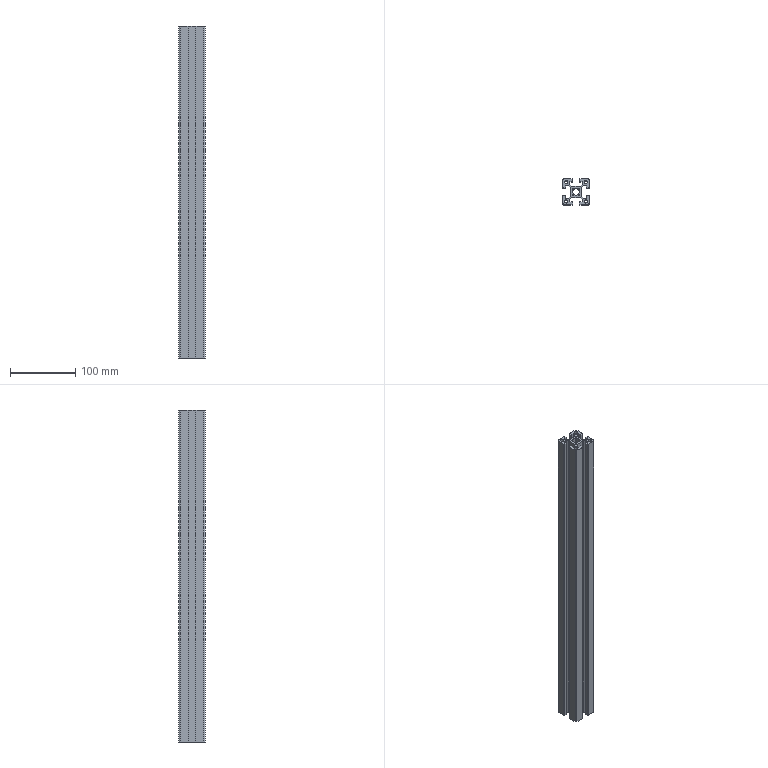Part | SolidWorks | features Extrusion 1 | 1 solid | 125 faces | box 40 x 40 x 510 mm | volume 357748 mm3 | plane 74 | cylinder 51 | commonest cylinder face diameters 2 x24 1.5 x10 5 x8 10.2 x5 4 x4